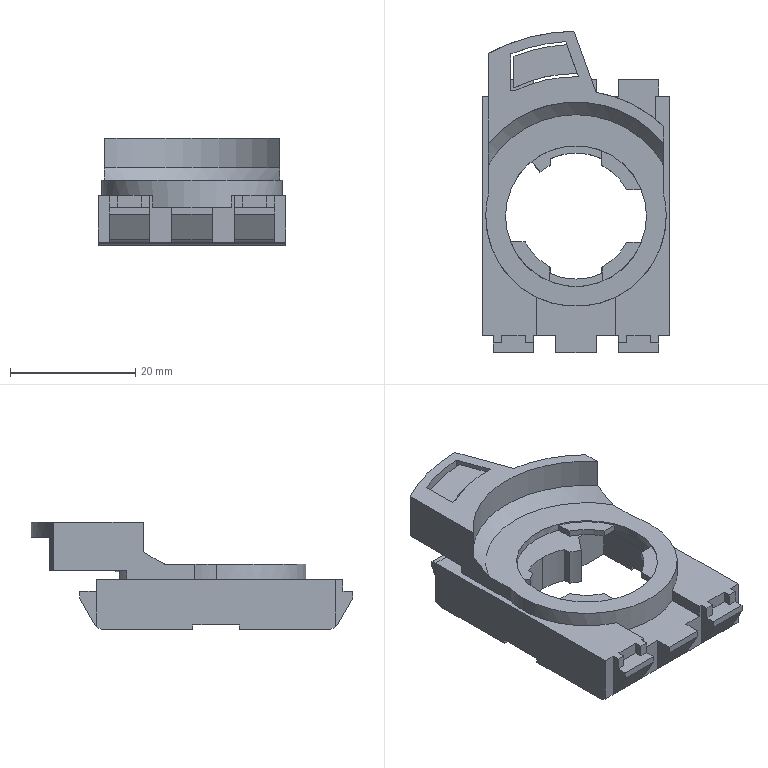Part | STEP file | A22NZ_H_02 | 1 solid | 170 faces | box 30 x 51.298 x 17.1 mm | volume 5133 mm3 | plane 141 | cylinder 27 | cone 2 | commonest cylinder face diameters 18.2 x7 20.1 x3 28.8 x3 4 x2 22.5 x2 25.4 x2